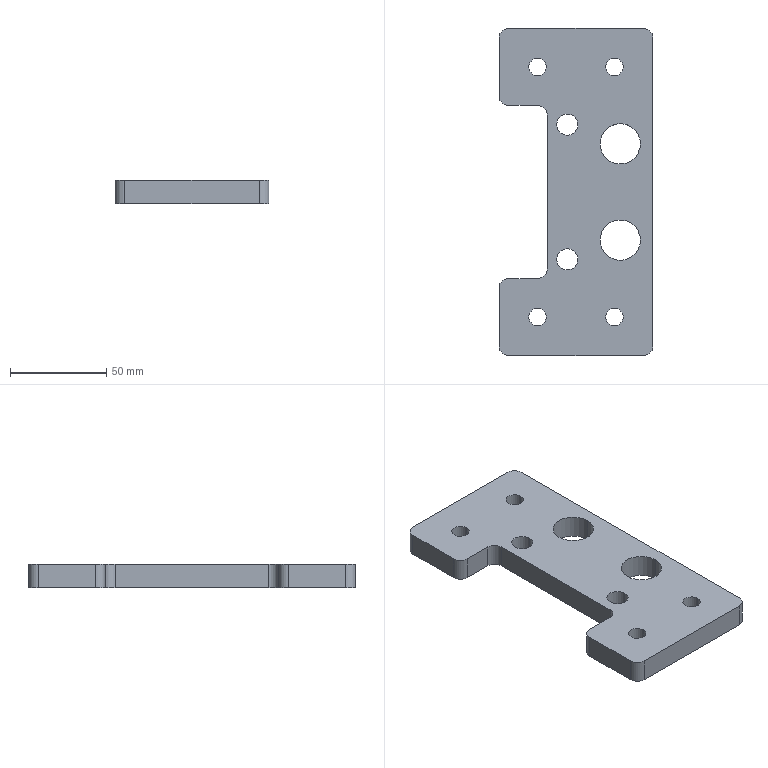Part | SolidWorks | features ICE 2, MoveFace 2, 3DProfileFeature 1, BaseBody 1, Fillet 1, HoleWzd 1 | 1 solid | 34 faces | box 80 x 170 x 12 mm | volume 122295 mm3 | cylinder 24 | plane 10 | commonest cylinder face diameters 9 x8 10 x8 11 x4 21 x4
STEP:
#1=CARTESIAN_POINT('',(33.5,25.,0.));
#2=VERTEX_POINT('',#1);
#3=CARTESIAN_POINT('',(12.5,25.,0.));
#4=VERTEX_POINT('',#3);
#5=CARTESIAN_POINT('',(23.,25.,0.));
#6=DIRECTION('',(0.,0.,-1.));
#7=DIRECTION('',(1.,0.,0.));
#8=AXIS2_PLACEMENT_3D('',#5,#6,#7);
#9=CIRCLE('',#8,10.5);
#10=EDGE_CURVE('',#2,#4,#9,.T.);
#11=ORIENTED_EDGE('',*,*,#10,.T.);
#12=CARTESIAN_POINT('',(12.5,25.,12.));
#13=VERTEX_POINT('',#12);
#14=CARTESIAN_POINT('',(12.5,25.,-0.001));
#15=DIRECTION('',(0.,0.,1.));
#16=VECTOR('',#15,1000.);
#17=LINE('',#14,#16);
#18=EDGE_CURVE('',#4,#13,#17,.T.);
#19=ORIENTED_EDGE('',*,*,#18,.T.);
#20=CARTESIAN_POINT('',(33.5,25.,12.));
#21=VERTEX_POINT('',#20);
#22=CARTESIAN_POINT('',(23.,25.,12.));
#23=DIRECTION('',(0.,0.,1.));
#24=DIRECTION('',(1.,0.,0.));
#25=AXIS2_PLACEMENT_3D('',#22,#23,#24);
#26=CIRCLE('',#25,10.5);
#27=EDGE_CURVE('',#13,#21,#26,.T.);
#28=ORIENTED_EDGE('',*,*,#27,.T.);
#29=CARTESIAN_POINT('',(33.5,25.,-0.001));
#30=DIRECTION('',(0.,0.,1.));
#31=VECTOR('',#30,1000.);
#32=LINE('',#29,#31);
#33=EDGE_CURVE('',#2,#21,#32,.T.);
#34=ORIENTED_EDGE('',*,*,#33,.F.);
#35=EDGE_LOOP('',(#11,#19,#28,#34));
#36=FACE_OUTER_BOUND('',#35,.T.);
#37=CARTESIAN_POINT('',(23.,25.,-0.001));
#38=DIRECTION('',(0.,0.,1.));
#39=DIRECTION('',(1.,0.,0.));
#40=AXIS2_PLACEMENT_3D('',#37,#38,#39);
#41=CYLINDRICAL_SURFACE('',#40,10.5);
#42=ADVANCED_FACE('',(#36),#41,.F.);
#43=CARTESIAN_POINT('',(33.5,-25.,0.));
#44=VERTEX_POINT('',#43);
#45=CARTESIAN_POINT('',(12.5,-25.,0.));
#46=VERTEX_POINT('',#45);
#47=CARTESIAN_POINT('',(23.,-25.,0.));
#48=DIRECTION('',(0.,0.,-1.));
#49=DIRECTION('',(1.,0.,0.));
#50=AXIS2_PLACEMENT_3D('',#47,#48,#49);
#51=CIRCLE('',#50,10.5);
#52=EDGE_CURVE('',#44,#46,#51,.T.);
#53=ORIENTED_EDGE('',*,*,#52,.T.);
#54=CARTESIAN_POINT('',(12.5,-25.,12.));
#55=VERTEX_POINT('',#54);
#56=CARTESIAN_POINT('',(12.5,-25.,-0.001));
#57=DIRECTION('',(0.,0.,1.));
#58=VECTOR('',#57,1000.);
#59=LINE('',#56,#58);
#60=EDGE_CURVE('',#46,#55,#59,.T.);
#61=ORIENTED_EDGE('',*,*,#60,.T.);
#62=CARTESIAN_POINT('',(33.5,-25.,12.));
#63=VERTEX_POINT('',#62);
#64=CARTESIAN_POINT('',(23.,-25.,12.));
#65=DIRECTION('',(0.,0.,1.));
#66=DIRECTION('',(1.,0.,0.));
#67=AXIS2_PLACEMENT_3D('',#64,#65,#66);
#68=CIRCLE('',#67,10.5);
#69=EDGE_CURVE('',#55,#63,#68,.T.);
#70=ORIENTED_EDGE('',*,*,#69,.T.);
#71=CARTESIAN_POINT('',(33.5,-25.,-0.001));
#72=DIRECTION('',(0.,0.,1.));
#73=VECTOR('',#72,1000.);
#74=LINE('',#71,#73);
#75=EDGE_CURVE('',#44,#63,#74,.T.);
#76=ORIENTED_EDGE('',*,*,#75,.F.);
#77=EDGE_LOOP('',(#53,#61,#70,#76));
#78=FACE_OUTER_BOUND('',#77,.T.);
#79=CARTESIAN_POINT('',(23.,-25.,-0.001));
#80=DIRECTION('',(0.,0.,1.));
#81=DIRECTION('',(1.,0.,0.));
#82=AXIS2_PLACEMENT_3D('',#79,#80,#81);
#83=CYLINDRICAL_SURFACE('',#82,10.5);
#84=ADVANCED_FACE('',(#78),#83,.F.);
#85=CARTESIAN_POINT('',(-10.,35.,0.));
#86=VERTEX_POINT('',#85);
#87=CARTESIAN_POINT('',(1.,35.,0.));
#88=VERTEX_POINT('',#87);
#89=CARTESIAN_POINT('',(-4.5,35.,0.));
#90=DIRECTION('',(0.,0.,1.));
#91=DIRECTION('',(1.,0.,0.));
#92=AXIS2_PLACEMENT_3D('',#89,#90,#91);
#93=CIRCLE('',#92,5.5);
#94=EDGE_CURVE('',#86,#88,#93,.T.);
#95=ORIENTED_EDGE('',*,*,#94,.F.);
#96=CARTESIAN_POINT('',(-10.,35.,12.));
#97=VERTEX_POINT('',#96);
#98=CARTESIAN_POINT('',(-10.,35.,10.));
#99=DIRECTION('',(0.,0.,1.));
#100=VECTOR('',#99,1000.);
#101=LINE('',#98,#100);
#102=EDGE_CURVE('',#86,#97,#101,.T.);
#103=ORIENTED_EDGE('',*,*,#102,.T.);
#104=CARTESIAN_POINT('',(1.,35.,12.));
#105=VERTEX_POINT('',#104);
#106=CARTESIAN_POINT('',(-4.5,35.,12.));
#107=DIRECTION('',(0.,0.,1.));
#108=DIRECTION('',(1.,0.,0.));
#109=AXIS2_PLACEMENT_3D('',#106,#107,#108);
#110=CIRCLE('',#109,5.5);
#111=EDGE_CURVE('',#97,#105,#110,.T.);
#112=ORIENTED_EDGE('',*,*,#111,.T.);
#113=CARTESIAN_POINT('',(1.,35.,10.));
#114=DIRECTION('',(0.,0.,1.));
#115=VECTOR('',#114,1000.);
#116=LINE('',#113,#115);
#117=EDGE_CURVE('',#88,#105,#116,.T.);
#118=ORIENTED_EDGE('',*,*,#117,.F.);
#119=EDGE_LOOP('',(#95,#103,#112,#118));
#120=FACE_OUTER_BOUND('',#119,.T.);
#121=CARTESIAN_POINT('',(-4.5,35.,10.));
#122=DIRECTION('',(0.,0.,1.));
#123=DIRECTION('',(1.,0.,0.));
#124=AXIS2_PLACEMENT_3D('',#121,#122,#123);
#125=CYLINDRICAL_SURFACE('',#124,5.5);
#126=ADVANCED_FACE('',(#120),#125,.F.);
#127=CARTESIAN_POINT('',(-10.,-35.,0.));
#128=VERTEX_POINT('',#127);
#129=CARTESIAN_POINT('',(1.,-35.,0.));
#130=VERTEX_POINT('',#129);
#131=CARTESIAN_POINT('',(-4.5,-35.,0.));
#132=DIRECTION('',(0.,0.,1.));
#133=DIRECTION('',(1.,0.,0.));
#134=AXIS2_PLACEMENT_3D('',#131,#132,#133);
#135=CIRCLE('',#134,5.5);
#136=EDGE_CURVE('',#128,#130,#135,.T.);
#137=ORIENTED_EDGE('',*,*,#136,.F.);
#138=CARTESIAN_POINT('',(-10.,-35.,12.));
#139=VERTEX_POINT('',#138);
#140=CARTESIAN_POINT('',(-10.,-35.,10.));
#141=DIRECTION('',(0.,0.,1.));
#142=VECTOR('',#141,1000.);
#143=LINE('',#140,#142);
#144=EDGE_CURVE('',#128,#139,#143,.T.);
#145=ORIENTED_EDGE('',*,*,#144,.T.);
#146=CARTESIAN_POINT('',(1.,-35.,12.));
#147=VERTEX_POINT('',#146);
#148=CARTESIAN_POINT('',(-4.5,-35.,12.));
#149=DIRECTION('',(0.,0.,1.));
#150=DIRECTION('',(1.,0.,0.));
#151=AXIS2_PLACEMENT_3D('',#148,#149,#150);
#152=CIRCLE('',#151,5.5);
#153=EDGE_CURVE('',#139,#147,#152,.T.);
#154=ORIENTED_EDGE('',*,*,#153,.T.);
#155=CARTESIAN_POINT('',(1.,-35.,10.));
#156=DIRECTION('',(0.,0.,1.));
#157=VECTOR('',#156,1000.);
#158=LINE('',#155,#157);
#159=EDGE_CURVE('',#130,#147,#158,.T.);
#160=ORIENTED_EDGE('',*,*,#159,.F.);
#161=EDGE_LOOP('',(#137,#145,#154,#160));
#162=FACE_OUTER_BOUND('',#161,.T.);
#163=CARTESIAN_POINT('',(-4.5,-35.,10.));
#164=DIRECTION('',(0.,0.,1.));
#165=DIRECTION('',(1.,0.,0.));
#166=AXIS2_PLACEMENT_3D('',#163,#164,#165);
#167=CYLINDRICAL_SURFACE('',#166,5.5);
#168=ADVANCED_FACE('',(#162),#167,.F.);
#169=CARTESIAN_POINT('',(-24.5,65.,0.));
#170=VERTEX_POINT('',#169);
#171=CARTESIAN_POINT('',(-15.5,65.,0.));
#172=VERTEX_POINT('',#171);
#173=CARTESIAN_POINT('',(-20.,65.,0.));
#174=DIRECTION('',(0.,0.,1.));
#175=DIRECTION('',(1.,0.,0.));
#176=AXIS2_PLACEMENT_3D('',#173,#174,#175);
#177=CIRCLE('',#176,4.5);
#178=EDGE_CURVE('',#170,#172,#177,.T.);
#179=ORIENTED_EDGE('',*,*,#178,.F.);
#180=CARTESIAN_POINT('',(-24.5,65.,12.));
#181=VERTEX_POINT('',#180);
#182=CARTESIAN_POINT('',(-24.5,65.,10.));
#183=DIRECTION('',(0.,0.,1.));
#184=VECTOR('',#183,1000.);
#185=LINE('',#182,#184);
#186=EDGE_CURVE('',#170,#181,#185,.T.);
#187=ORIENTED_EDGE('',*,*,#186,.T.);
#188=CARTESIAN_POINT('',(-15.5,65.,12.));
#189=VERTEX_POINT('',#188);
#190=CARTESIAN_POINT('',(-20.,65.,12.));
#191=DIRECTION('',(0.,0.,1.));
#192=DIRECTION('',(1.,0.,0.));
#193=AXIS2_PLACEMENT_3D('',#190,#191,#192);
#194=CIRCLE('',#193,4.5);
#195=EDGE_CURVE('',#181,#189,#194,.T.);
#196=ORIENTED_EDGE('',*,*,#195,.T.);
#197=CARTESIAN_POINT('',(-15.5,65.,10.));
#198=DIRECTION('',(0.,0.,1.));
#199=VECTOR('',#198,1000.);
#200=LINE('',#197,#199);
#201=EDGE_CURVE('',#172,#189,#200,.T.);
#202=ORIENTED_EDGE('',*,*,#201,.F.);
#203=EDGE_LOOP('',(#179,#187,#196,#202));
#204=FACE_OUTER_BOUND('',#203,.T.);
#205=CARTESIAN_POINT('',(-20.,65.,10.));
#206=DIRECTION('',(0.,0.,1.));
#207=DIRECTION('',(1.,0.,0.));
#208=AXIS2_PLACEMENT_3D('',#205,#206,#207);
#209=CYLINDRICAL_SURFACE('',#208,4.5);
#210=ADVANCED_FACE('',(#204),#209,.F.);
#211=CARTESIAN_POINT('',(15.5,65.,0.));
#212=VERTEX_POINT('',#211);
#213=CARTESIAN_POINT('',(24.5,65.,0.));
#214=VERTEX_POINT('',#213);
#215=CARTESIAN_POINT('',(20.,65.,0.));
#216=DIRECTION('',(0.,0.,1.));
#217=DIRECTION('',(1.,0.,0.));
#218=AXIS2_PLACEMENT_3D('',#215,#216,#217);
#219=CIRCLE('',#218,4.5);
#220=EDGE_CURVE('',#212,#214,#219,.T.);
#221=ORIENTED_EDGE('',*,*,#220,.F.);
#222=CARTESIAN_POINT('',(15.5,65.,12.));
#223=VERTEX_POINT('',#222);
#224=CARTESIAN_POINT('',(15.5,65.,10.));
#225=DIRECTION('',(0.,0.,1.));
#226=VECTOR('',#225,1000.);
#227=LINE('',#224,#226);
#228=EDGE_CURVE('',#212,#223,#227,.T.);
#229=ORIENTED_EDGE('',*,*,#228,.T.);
#230=CARTESIAN_POINT('',(24.5,65.,12.));
#231=VERTEX_POINT('',#230);
#232=CARTESIAN_POINT('',(20.,65.,12.));
#233=DIRECTION('',(0.,0.,1.));
#234=DIRECTION('',(1.,0.,0.));
#235=AXIS2_PLACEMENT_3D('',#232,#233,#234);
#236=CIRCLE('',#235,4.5);
#237=EDGE_CURVE('',#223,#231,#236,.T.);
#238=ORIENTED_EDGE('',*,*,#237,.T.);
#239=CARTESIAN_POINT('',(24.5,65.,10.));
#240=DIRECTION('',(0.,0.,1.));
#241=VECTOR('',#240,1000.);
#242=LINE('',#239,#241);
#243=EDGE_CURVE('',#214,#231,#242,.T.);
#244=ORIENTED_EDGE('',*,*,#243,.F.);
#245=EDGE_LOOP('',(#221,#229,#238,#244));
#246=FACE_OUTER_BOUND('',#245,.T.);
#247=CARTESIAN_POINT('',(20.,65.,10.));
#248=DIRECTION('',(0.,0.,1.));
#249=DIRECTION('',(1.,0.,0.));
#250=AXIS2_PLACEMENT_3D('',#247,#248,#249);
#251=CYLINDRICAL_SURFACE('',#250,4.5);
#252=ADVANCED_FACE('',(#246),#251,.F.);
#253=CARTESIAN_POINT('',(-24.5,-65.,0.));
#254=VERTEX_POINT('',#253);
#255=CARTESIAN_POINT('',(-15.5,-65.,0.));
#256=VERTEX_POINT('',#255);
#257=CARTESIAN_POINT('',(-20.,-65.,0.));
#258=DIRECTION('',(0.,0.,1.));
#259=DIRECTION('',(1.,0.,0.));
#260=AXIS2_PLACEMENT_3D('',#257,#258,#259);
#261=CIRCLE('',#260,4.5);
#262=EDGE_CURVE('',#254,#256,#261,.T.);
#263=ORIENTED_EDGE('',*,*,#262,.F.);
#264=CARTESIAN_POINT('',(-24.5,-65.,12.));
#265=VERTEX_POINT('',#264);
#266=CARTESIAN_POINT('',(-24.5,-65.,10.));
#267=DIRECTION('',(0.,0.,1.));
#268=VECTOR('',#267,1000.);
#269=LINE('',#266,#268);
#270=EDGE_CURVE('',#254,#265,#269,.T.);
#271=ORIENTED_EDGE('',*,*,#270,.T.);
#272=CARTESIAN_POINT('',(-15.5,-65.,12.));
#273=VERTEX_POINT('',#272);
#274=CARTESIAN_POINT('',(-20.,-65.,12.));
#275=DIRECTION('',(0.,0.,1.));
#276=DIRECTION('',(1.,0.,0.));
#277=AXIS2_PLACEMENT_3D('',#274,#275,#276);
#278=CIRCLE('',#277,4.5);
#279=EDGE_CURVE('',#265,#273,#278,.T.);
#280=ORIENTED_EDGE('',*,*,#279,.T.);
#281=CARTESIAN_POINT('',(-15.5,-65.,10.));
#282=DIRECTION('',(0.,0.,1.));
#283=VECTOR('',#282,1000.);
#284=LINE('',#281,#283);
#285=EDGE_CURVE('',#256,#273,#284,.T.);
#286=ORIENTED_EDGE('',*,*,#285,.F.);
#287=EDGE_LOOP('',(#263,#271,#280,#286));
#288=FACE_OUTER_BOUND('',#287,.T.);
#289=CARTESIAN_POINT('',(-20.,-65.,10.));
#290=DIRECTION('',(0.,0.,1.));
#291=DIRECTION('',(1.,0.,0.));
#292=AXIS2_PLACEMENT_3D('',#289,#290,#291);
#293=CYLINDRICAL_SURFACE('',#292,4.5);
#294=ADVANCED_FACE('',(#288),#293,.F.);
#295=CARTESIAN_POINT('',(15.5,-65.,0.));
#296=VERTEX_POINT('',#295);
#297=CARTESIAN_POINT('',(24.5,-65.,0.));
#298=VERTEX_POINT('',#297);
#299=CARTESIAN_POINT('',(20.,-65.,0.));
#300=DIRECTION('',(0.,0.,1.));
#301=DIRECTION('',(1.,0.,0.));
#302=AXIS2_PLACEMENT_3D('',#299,#300,#301);
#303=CIRCLE('',#302,4.5);
#304=EDGE_CURVE('',#296,#298,#303,.T.);
#305=ORIENTED_EDGE('',*,*,#304,.F.);
#306=CARTESIAN_POINT('',(15.5,-65.,12.));
#307=VERTEX_POINT('',#306);
#308=CARTESIAN_POINT('',(15.5,-65.,10.));
#309=DIRECTION('',(0.,0.,1.));
#310=VECTOR('',#309,1000.);
#311=LINE('',#308,#310);
#312=EDGE_CURVE('',#296,#307,#311,.T.);
#313=ORIENTED_EDGE('',*,*,#312,.T.);
#314=CARTESIAN_POINT('',(24.5,-65.,12.));
#315=VERTEX_POINT('',#314);
#316=CARTESIAN_POINT('',(20.,-65.,12.));
#317=DIRECTION('',(0.,0.,1.));
#318=DIRECTION('',(1.,0.,0.));
#319=AXIS2_PLACEMENT_3D('',#316,#317,#318);
#320=CIRCLE('',#319,4.5);
#321=EDGE_CURVE('',#307,#315,#320,.T.);
#322=ORIENTED_EDGE('',*,*,#321,.T.);
#323=CARTESIAN_POINT('',(24.5,-65.,10.));
#324=DIRECTION('',(0.,0.,1.));
#325=VECTOR('',#324,1000.);
#326=LINE('',#323,#325);
#327=EDGE_CURVE('',#298,#315,#326,.T.);
#328=ORIENTED_EDGE('',*,*,#327,.F.);
#329=EDGE_LOOP('',(#305,#313,#322,#328));
#330=FACE_OUTER_BOUND('',#329,.T.);
#331=CARTESIAN_POINT('',(20.,-65.,10.));
#332=DIRECTION('',(0.,0.,1.));
#333=DIRECTION('',(1.,0.,0.));
#334=AXIS2_PLACEMENT_3D('',#331,#332,#333);
#335=CYLINDRICAL_SURFACE('',#334,4.5);
#336=ADVANCED_FACE('',(#330),#335,.F.);
#337=CARTESIAN_POINT('',(-40.,80.,0.));
#338=VERTEX_POINT('',#337);
#339=CARTESIAN_POINT('',(-40.,50.,0.));
#340=VERTEX_POINT('',#339);
#341=CARTESIAN_POINT('',(-40.,85.,0.));
#342=DIRECTION('',(0.,-1.,0.));
#343=VECTOR('',#342,1000.);
#344=LINE('',#341,#343);
#345=EDGE_CURVE('',#338,#340,#344,.T.);
#346=ORIENTED_EDGE('',*,*,#345,.T.);
#347=CARTESIAN_POINT('',(-40.,50.,12.));
#348=VERTEX_POINT('',#347);
#349=CARTESIAN_POINT('',(-40.,50.,10.));
#350=DIRECTION('',(0.,0.,1.));
#351=VECTOR('',#350,1000.);
#352=LINE('',#349,#351);
#353=EDGE_CURVE('',#340,#348,#352,.T.);
#354=ORIENTED_EDGE('',*,*,#353,.T.);
#355=CARTESIAN_POINT('',(-40.,80.,12.));
#356=VERTEX_POINT('',#355);
#357=CARTESIAN_POINT('',(-40.,85.,12.));
#358=DIRECTION('',(0.,-1.,0.));
#359=VECTOR('',#358,1000.);
#360=LINE('',#357,#359);
#361=EDGE_CURVE('',#356,#348,#360,.T.);
#362=ORIENTED_EDGE('',*,*,#361,.F.);
#363=CARTESIAN_POINT('',(-40.,80.,10.));
#364=DIRECTION('',(0.,0.,-1.));
#365=VECTOR('',#364,1000.);
#366=LINE('',#363,#365);
#367=EDGE_CURVE('',#356,#338,#366,.T.);
#368=ORIENTED_EDGE('',*,*,#367,.T.);
#369=EDGE_LOOP('',(#346,#354,#362,#368));
#370=FACE_OUTER_BOUND('',#369,.T.);
#371=CARTESIAN_POINT('',(-40.,85.,10.));
#372=DIRECTION('',(1.,0.,0.));
#373=DIRECTION('',(0.,1.,0.));
#374=AXIS2_PLACEMENT_3D('',#371,#372,#373);
#375=PLANE('',#374);
#376=ADVANCED_FACE('',(#370),#375,.F.);
#377=CARTESIAN_POINT('',(-35.,85.,12.));
#378=VERTEX_POINT('',#377);
#379=CARTESIAN_POINT('',(-35.,80.,12.));
#380=DIRECTION('',(0.,0.,1.));
#381=DIRECTION('',(1.,0.,0.));
#382=AXIS2_PLACEMENT_3D('',#379,#380,#381);
#383=CIRCLE('',#382,5.);
#384=EDGE_CURVE('',#378,#356,#383,.T.);
#385=ORIENTED_EDGE('',*,*,#384,.F.);
#386=CARTESIAN_POINT('',(-35.,85.,0.));
#387=VERTEX_POINT('',#386);
#388=CARTESIAN_POINT('',(-35.,85.,10.));
#389=DIRECTION('',(0.,0.,1.));
#390=VECTOR('',#389,1000.);
#391=LINE('',#388,#390);
#392=EDGE_CURVE('',#387,#378,#391,.T.);
#393=ORIENTED_EDGE('',*,*,#392,.F.);
#394=CARTESIAN_POINT('',(-35.,80.,0.));
#395=DIRECTION('',(0.,0.,-1.));
#396=DIRECTION('',(1.,0.,0.));
#397=AXIS2_PLACEMENT_3D('',#394,#395,#396);
#398=CIRCLE('',#397,5.);
#399=EDGE_CURVE('',#338,#387,#398,.T.);
#400=ORIENTED_EDGE('',*,*,#399,.F.);
#401=ORIENTED_EDGE('',*,*,#367,.F.);
#402=EDGE_LOOP('',(#385,#393,#400,#401));
#403=FACE_OUTER_BOUND('',#402,.T.);
#404=CARTESIAN_POINT('',(-35.,80.,10.));
#405=DIRECTION('',(0.,0.,-1.));
#406=DIRECTION('',(-1.,0.,0.));
#407=AXIS2_PLACEMENT_3D('',#404,#405,#406);
#408=CYLINDRICAL_SURFACE('',#407,5.);
#409=ADVANCED_FACE('',(#403),#408,.T.);
#410=CARTESIAN_POINT('',(40.,80.,12.));
#411=VERTEX_POINT('',#410);
#412=CARTESIAN_POINT('',(35.,85.,12.));
#413=VERTEX_POINT('',#412);
#414=CARTESIAN_POINT('',(35.,80.,12.));
#415=DIRECTION('',(0.,0.,1.));
#416=DIRECTION('',(1.,0.,0.));
#417=AXIS2_PLACEMENT_3D('',#414,#415,#416);
#418=CIRCLE('',#417,5.);
#419=EDGE_CURVE('',#411,#413,#418,.T.);
#420=ORIENTED_EDGE('',*,*,#419,.F.);
#421=CARTESIAN_POINT('',(40.,80.,0.));
#422=VERTEX_POINT('',#421);
#423=CARTESIAN_POINT('',(40.,80.,10.));
#424=DIRECTION('',(0.,0.,1.));
#425=VECTOR('',#424,1000.);
#426=LINE('',#423,#425);
#427=EDGE_CURVE('',#422,#411,#426,.T.);
#428=ORIENTED_EDGE('',*,*,#427,.F.);
#429=CARTESIAN_POINT('',(35.,85.,0.));
#430=VERTEX_POINT('',#429);
#431=CARTESIAN_POINT('',(35.,80.,0.));
#432=DIRECTION('',(0.,0.,-1.));
#433=DIRECTION('',(1.,0.,0.));
#434=AXIS2_PLACEMENT_3D('',#431,#432,#433);
#435=CIRCLE('',#434,5.);
#436=EDGE_CURVE('',#430,#422,#435,.T.);
#437=ORIENTED_EDGE('',*,*,#436,.F.);
#438=CARTESIAN_POINT('',(35.,85.,10.));
#439=DIRECTION('',(0.,0.,-1.));
#440=VECTOR('',#439,1000.);
#441=LINE('',#438,#440);
#442=EDGE_CURVE('',#413,#430,#441,.T.);
#443=ORIENTED_EDGE('',*,*,#442,.F.);
#444=EDGE_LOOP('',(#420,#428,#437,#443));
#445=FACE_OUTER_BOUND('',#444,.T.);
#446=CARTESIAN_POINT('',(35.,80.,10.));
#447=DIRECTION('',(0.,0.,-1.));
#448=DIRECTION('',(-1.,0.,0.));
#449=AXIS2_PLACEMENT_3D('',#446,#447,#448);
#450=CYLINDRICAL_SURFACE('',#449,5.);
#451=ADVANCED_FACE('',(#445),#450,.T.);
#452=CARTESIAN_POINT('',(35.,-85.,12.));
#453=VERTEX_POINT('',#452);
#454=CARTESIAN_POINT('',(40.,-80.,12.));
#455=VERTEX_POINT('',#454);
#456=CARTESIAN_POINT('',(35.,-80.,12.));
#457=DIRECTION('',(0.,0.,1.));
#458=DIRECTION('',(1.,0.,0.));
#459=AXIS2_PLACEMENT_3D('',#456,#457,#458);
#460=CIRCLE('',#459,5.);
#461=EDGE_CURVE('',#453,#455,#460,.T.);
#462=ORIENTED_EDGE('',*,*,#461,.F.);
#463=CARTESIAN_POINT('',(35.,-85.,0.));
#464=VERTEX_POINT('',#463);
#465=CARTESIAN_POINT('',(35.,-85.,10.));
#466=DIRECTION('',(0.,0.,1.));
#467=VECTOR('',#466,1000.);
#468=LINE('',#465,#467);
#469=EDGE_CURVE('',#464,#453,#468,.T.);
#470=ORIENTED_EDGE('',*,*,#469,.F.);
#471=CARTESIAN_POINT('',(40.,-80.,0.));
#472=VERTEX_POINT('',#471);
#473=CARTESIAN_POINT('',(35.,-80.,0.));
#474=DIRECTION('',(0.,0.,-1.));
#475=DIRECTION('',(1.,0.,0.));
#476=AXIS2_PLACEMENT_3D('',#473,#474,#475);
#477=CIRCLE('',#476,5.);
#478=EDGE_CURVE('',#472,#464,#477,.T.);
#479=ORIENTED_EDGE('',*,*,#478,.F.);
#480=CARTESIAN_POINT('',(40.,-80.,10.));
#481=DIRECTION('',(0.,0.,-1.));
#482=VECTOR('',#481,1000.);
#483=LINE('',#480,#482);
#484=EDGE_CURVE('',#455,#472,#483,.T.);
#485=ORIENTED_EDGE('',*,*,#484,.F.);
#486=EDGE_LOOP('',(#462,#470,#479,#485));
#487=FACE_OUTER_BOUND('',#486,.T.);
#488=CARTESIAN_POINT('',(35.,-80.,10.));
#489=DIRECTION('',(0.,0.,-1.));
#490=DIRECTION('',(-1.,0.,0.));
#491=AXIS2_PLACEMENT_3D('',#488,#489,#490);
#492=CYLINDRICAL_SURFACE('',#491,5.);
#493=ADVANCED_FACE('',(#487),#492,.T.);
#494=CARTESIAN_POINT('',(-40.,-80.,12.));
#495=VERTEX_POINT('',#494);
#496=CARTESIAN_POINT('',(-35.,-85.,12.));
#497=VERTEX_POINT('',#496);
#498=CARTESIAN_POINT('',(-35.,-80.,12.));
#499=DIRECTION('',(0.,0.,1.));
#500=DIRECTION('',(1.,0.,0.));
#501=AXIS2_PLACEMENT_3D('',#498,#499,#500);
#502=CIRCLE('',#501,5.);
#503=EDGE_CURVE('',#495,#497,#502,.T.);
#504=ORIENTED_EDGE('',*,*,#503,.F.);
#505=CARTESIAN_POINT('',(-40.,-80.,0.));
#506=VERTEX_POINT('',#505);
#507=CARTESIAN_POINT('',(-40.,-80.,10.));
#508=DIRECTION('',(0.,0.,1.));
#509=VECTOR('',#508,1000.);
#510=LINE('',#507,#509);
#511=EDGE_CURVE('',#506,#495,#510,.T.);
#512=ORIENTED_EDGE('',*,*,#511,.F.);
#513=CARTESIAN_POINT('',(-35.,-85.,0.));
#514=VERTEX_POINT('',#513);
#515=CARTESIAN_POINT('',(-35.,-80.,0.));
#516=DIRECTION('',(0.,0.,-1.));
#517=DIRECTION('',(1.,0.,0.));
#518=AXIS2_PLACEMENT_3D('',#515,#516,#517);
#519=CIRCLE('',#518,5.);
#520=EDGE_CURVE('',#514,#506,#519,.T.);
#521=ORIENTED_EDGE('',*,*,#520,.F.);
#522=CARTESIAN_POINT('',(-35.,-85.,10.));
#523=DIRECTION('',(0.,0.,-1.));
#524=VECTOR('',#523,1000.);
#525=LINE('',#522,#524);
#526=EDGE_CURVE('',#497,#514,#525,.T.);
#527=ORIENTED_EDGE('',*,*,#526,.F.);
#528=EDGE_LOOP('',(#504,#512,#521,#527));
#529=FACE_OUTER_BOUND('',#528,.T.);
#530=CARTESIAN_POINT('',(-35.,-80.,10.));
#531=DIRECTION('',(0.,0.,-1.));
#532=DIRECTION('',(-1.,0.,0.));
#533=AXIS2_PLACEMENT_3D('',#530,#531,#532);
#534=CYLINDRICAL_SURFACE('',#533,5.);
#535=ADVANCED_FACE('',(#529),#534,.T.);
#536=ORIENTED_EDGE('',*,*,#10,.F.);
#537=CARTESIAN_POINT('',(23.,25.,0.));
#538=DIRECTION('',(0.,0.,-1.));
#539=DIRECTION('',(1.,0.,0.));
#540=AXIS2_PLACEMENT_3D('',#537,#538,#539);
#541=CIRCLE('',#540,10.5);
#542=EDGE_CURVE('',#4,#2,#541,.T.);
#543=ORIENTED_EDGE('',*,*,#542,.F.);
#544=EDGE_LOOP('',(#536,#543));
#545=FACE_BOUND('',#544,.T.);
#546=ORIENTED_EDGE('',*,*,#52,.F.);
#547=CARTESIAN_POINT('',(23.,-25.,0.));
#548=DIRECTION('',(0.,0.,-1.));
#549=DIRECTION('',(1.,0.,0.));
#550=AXIS2_PLACEMENT_3D('',#547,#548,#549);
#551=CIRCLE('',#550,10.5);
#552=EDGE_CURVE('',#46,#44,#551,.T.);
#553=ORIENTED_EDGE('',*,*,#552,.F.);
#554=EDGE_LOOP('',(#546,#553));
#555=FACE_BOUND('',#554,.T.);
#556=CARTESIAN_POINT('',(20.,-65.,0.));
#557=DIRECTION('',(0.,0.,1.));
#558=DIRECTION('',(1.,0.,0.));
#559=AXIS2_PLACEMENT_3D('',#556,#557,#558);
#560=CIRCLE('',#559,4.5);
#561=EDGE_CURVE('',#298,#296,#560,.T.);
#562=ORIENTED_EDGE('',*,*,#561,.T.);
#563=ORIENTED_EDGE('',*,*,#304,.T.);
#564=EDGE_LOOP('',(#562,#563));
#565=FACE_BOUND('',#564,.T.);
#566=CARTESIAN_POINT('',(-20.,-65.,0.));
#567=DIRECTION('',(0.,0.,1.));
#568=DIRECTION('',(1.,0.,0.));
#569=AXIS2_PLACEMENT_3D('',#566,#567,#568);
#570=CIRCLE('',#569,4.5);
#571=EDGE_CURVE('',#256,#254,#570,.T.);
#572=ORIENTED_EDGE('',*,*,#571,.T.);
#573=ORIENTED_EDGE('',*,*,#262,.T.);
#574=EDGE_LOOP('',(#572,#573));
#575=FACE_BOUND('',#574,.T.);
#576=CARTESIAN_POINT('',(20.,65.,0.));
#577=DIRECTION('',(0.,0.,1.));
#578=DIRECTION('',(1.,0.,0.));
#579=AXIS2_PLACEMENT_3D('',#576,#577,#578);
#580=CIRCLE('',#579,4.5);
#581=EDGE_CURVE('',#214,#212,#580,.T.);
#582=ORIENTED_EDGE('',*,*,#581,.T.);
#583=ORIENTED_EDGE('',*,*,#220,.T.);
#584=EDGE_LOOP('',(#582,#583));
#585=FACE_BOUND('',#584,.T.);
#586=CARTESIAN_POINT('',(-20.,65.,0.));
#587=DIRECTION('',(0.,0.,1.));
#588=DIRECTION('',(1.,0.,0.));
#589=AXIS2_PLACEMENT_3D('',#586,#587,#588);
#590=CIRCLE('',#589,4.5);
#591=EDGE_CURVE('',#172,#170,#590,.T.);
#592=ORIENTED_EDGE('',*,*,#591,.T.);
#593=ORIENTED_EDGE('',*,*,#178,.T.);
#594=EDGE_LOOP('',(#592,#593));
#595=FACE_BOUND('',#594,.T.);
#596=CARTESIAN_POINT('',(-4.5,-35.,0.));
#597=DIRECTION('',(0.,0.,1.));
#598=DIRECTION('',(1.,0.,0.));
#599=AXIS2_PLACEMENT_3D('',#596,#597,#598);
#600=CIRCLE('',#599,5.5);
#601=EDGE_CURVE('',#130,#128,#600,.T.);
#602=ORIENTED_EDGE('',*,*,#601,.T.);
#603=ORIENTED_EDGE('',*,*,#136,.T.);
#604=EDGE_LOOP('',(#602,#603));
#605=FACE_BOUND('',#604,.T.);
#606=CARTESIAN_POINT('',(-4.5,35.,0.));
#607=DIRECTION('',(0.,0.,1.));
#608=DIRECTION('',(1.,0.,0.));
#609=AXIS2_PLACEMENT_3D('',#606,#607,#608);
#610=CIRCLE('',#609,5.5);
#611=EDGE_CURVE('',#88,#86,#610,.T.);
#612=ORIENTED_EDGE('',*,*,#611,.T.);
#613=ORIENTED_EDGE('',*,*,#94,.T.);
#614=EDGE_LOOP('',(#612,#613));
#615=FACE_BOUND('',#614,.T.);
#616=CARTESIAN_POINT('',(-40.,-50.,0.));
#617=VERTEX_POINT('',#616);
#618=CARTESIAN_POINT('',(-40.,85.,0.));
#619=DIRECTION('',(0.,-1.,0.));
#620=VECTOR('',#619,1000.);
#621=LINE('',#618,#620);
#622=EDGE_CURVE('',#617,#506,#621,.T.);
#623=ORIENTED_EDGE('',*,*,#622,.F.);
#624=CARTESIAN_POINT('',(-35.,-45.,0.));
#625=VERTEX_POINT('',#624);
#626=CARTESIAN_POINT('',(-35.,-50.,0.));
#627=DIRECTION('',(0.,0.,-1.));
#628=DIRECTION('',(1.,0.,0.));
#629=AXIS2_PLACEMENT_3D('',#626,#627,#628);
#630=CIRCLE('',#629,5.);
#631=EDGE_CURVE('',#617,#625,#630,.T.);
#632=ORIENTED_EDGE('',*,*,#631,.T.);
#633=CARTESIAN_POINT('',(-20.,-45.,0.));
#634=VERTEX_POINT('',#633);
#635=CARTESIAN_POINT('',(-15.,-45.,0.));
#636=DIRECTION('',(-1.,0.,0.));
#637=VECTOR('',#636,1000.);
#638=LINE('',#635,#637);
#639=EDGE_CURVE('',#634,#625,#638,.T.);
#640=ORIENTED_EDGE('',*,*,#639,.F.);
#641=CARTESIAN_POINT('',(-15.,-40.,0.));
#642=VERTEX_POINT('',#641);
#643=CARTESIAN_POINT('',(-20.,-40.,0.));
#644=DIRECTION('',(0.,0.,1.));
#645=DIRECTION('',(1.,0.,0.));
#646=AXIS2_PLACEMENT_3D('',#643,#644,#645);
#647=CIRCLE('',#646,5.);
#648=EDGE_CURVE('',#634,#642,#647,.T.);
#649=ORIENTED_EDGE('',*,*,#648,.T.);
#650=CARTESIAN_POINT('',(-15.,40.,0.));
#651=VERTEX_POINT('',#650);
#652=CARTESIAN_POINT('',(-15.,45.,0.));
#653=DIRECTION('',(0.,-1.,0.));
#654=VECTOR('',#653,1000.);
#655=LINE('',#652,#654);
#656=EDGE_CURVE('',#651,#642,#655,.T.);
#657=ORIENTED_EDGE('',*,*,#656,.F.);
#658=CARTESIAN_POINT('',(-20.,45.,0.));
#659=VERTEX_POINT('',#658);
#660=CARTESIAN_POINT('',(-20.,40.,0.));
#661=DIRECTION('',(0.,0.,1.));
#662=DIRECTION('',(1.,0.,0.));
#663=AXIS2_PLACEMENT_3D('',#660,#661,#662);
#664=CIRCLE('',#663,5.);
#665=EDGE_CURVE('',#651,#659,#664,.T.);
#666=ORIENTED_EDGE('',*,*,#665,.T.);
#667=CARTESIAN_POINT('',(-35.,45.,0.));
#668=VERTEX_POINT('',#667);
#669=CARTESIAN_POINT('',(-40.,45.,0.));
#670=DIRECTION('',(1.,0.,0.));
#671=VECTOR('',#670,1000.);
#672=LINE('',#669,#671);
#673=EDGE_CURVE('',#668,#659,#672,.T.);
#674=ORIENTED_EDGE('',*,*,#673,.F.);
#675=CARTESIAN_POINT('',(-35.,50.,0.));
#676=DIRECTION('',(0.,0.,-1.));
#677=DIRECTION('',(1.,0.,0.));
#678=AXIS2_PLACEMENT_3D('',#675,#676,#677);
#679=CIRCLE('',#678,5.);
#680=EDGE_CURVE('',#668,#340,#679,.T.);
#681=ORIENTED_EDGE('',*,*,#680,.T.);
#682=ORIENTED_EDGE('',*,*,#345,.F.);
#683=ORIENTED_EDGE('',*,*,#399,.T.);
#684=CARTESIAN_POINT('',(-40.,85.,0.));
#685=DIRECTION('',(-1.,0.,0.));
#686=VECTOR('',#685,1000.);
#687=LINE('',#684,#686);
#688=EDGE_CURVE('',#430,#387,#687,.T.);
#689=ORIENTED_EDGE('',*,*,#688,.F.);
#690=ORIENTED_EDGE('',*,*,#436,.T.);
#691=CARTESIAN_POINT('',(40.,85.,0.));
#692=DIRECTION('',(0.,1.,0.));
#693=VECTOR('',#692,1000.);
#694=LINE('',#691,#693);
#695=EDGE_CURVE('',#472,#422,#694,.T.);
#696=ORIENTED_EDGE('',*,*,#695,.F.);
#697=ORIENTED_EDGE('',*,*,#478,.T.);
#698=CARTESIAN_POINT('',(-40.,-85.,0.));
#699=DIRECTION('',(1.,0.,0.));
#700=VECTOR('',#699,1000.);
#701=LINE('',#698,#700);
#702=EDGE_CURVE('',#514,#464,#701,.T.);
#703=ORIENTED_EDGE('',*,*,#702,.F.);
#704=ORIENTED_EDGE('',*,*,#520,.T.);
#705=EDGE_LOOP('',(#623,#632,#640,#649,#657,#666,#674,#681,#682,#683,#689,#690,#696,#697,#703,#704));
#706=FACE_OUTER_BOUND('',#705,.T.);
#707=CARTESIAN_POINT('',(0.,0.,0.));
#708=DIRECTION('',(0.,0.,1.));
#709=DIRECTION('',(1.,0.,0.));
#710=AXIS2_PLACEMENT_3D('',#707,#708,#709);
#711=PLANE('',#710);
#712=ADVANCED_FACE('',(#545,#555,#565,#575,#585,#595,#605,#615,#706),#711,.F.);
#713=CARTESIAN_POINT('',(23.,25.,12.));
#714=DIRECTION('',(0.,0.,1.));
#715=DIRECTION('',(1.,0.,0.));
#716=AXIS2_PLACEMENT_3D('',#713,#714,#715);
#717=CIRCLE('',#716,10.5);
#718=EDGE_CURVE('',#21,#13,#717,.T.);
#719=ORIENTED_EDGE('',*,*,#718,.F.);
#720=ORIENTED_EDGE('',*,*,#27,.F.);
#721=EDGE_LOOP('',(#719,#720));
#722=FACE_BOUND('',#721,.T.);
#723=CARTESIAN_POINT('',(23.,-25.,12.));
#724=DIRECTION('',(0.,0.,1.));
#725=DIRECTION('',(1.,0.,0.));
#726=AXIS2_PLACEMENT_3D('',#723,#724,#725);
#727=CIRCLE('',#726,10.5);
#728=EDGE_CURVE('',#63,#55,#727,.T.);
#729=ORIENTED_EDGE('',*,*,#728,.F.);
#730=ORIENTED_EDGE('',*,*,#69,.F.);
#731=EDGE_LOOP('',(#729,#730));
#732=FACE_BOUND('',#731,.T.);
#733=CARTESIAN_POINT('',(-35.,-45.,12.));
#734=VERTEX_POINT('',#733);
#735=CARTESIAN_POINT('',(-20.,-45.,12.));
#736=VERTEX_POINT('',#735);
#737=CARTESIAN_POINT('',(-15.,-45.,12.));
#738=DIRECTION('',(1.,0.,0.));
#739=VECTOR('',#738,1000.);
#740=LINE('',#737,#739);
#741=EDGE_CURVE('',#734,#736,#740,.T.);
#742=ORIENTED_EDGE('',*,*,#741,.F.);
#743=CARTESIAN_POINT('',(-40.,-50.,12.));
#744=VERTEX_POINT('',#743);
#745=CARTESIAN_POINT('',(-35.,-50.,12.));
#746=DIRECTION('',(0.,0.,1.));
#747=DIRECTION('',(1.,0.,0.));
#748=AXIS2_PLACEMENT_3D('',#745,#746,#747);
#749=CIRCLE('',#748,5.);
#750=EDGE_CURVE('',#734,#744,#749,.T.);
#751=ORIENTED_EDGE('',*,*,#750,.T.);
#752=CARTESIAN_POINT('',(-40.,85.,12.));
#753=DIRECTION('',(0.,-1.,0.));
#754=VECTOR('',#753,1000.);
#755=LINE('',#752,#754);
#756=EDGE_CURVE('',#744,#495,#755,.T.);
#757=ORIENTED_EDGE('',*,*,#756,.T.);
#758=ORIENTED_EDGE('',*,*,#503,.T.);
#759=CARTESIAN_POINT('',(-40.,-85.,12.));
#760=DIRECTION('',(1.,0.,0.));
#761=VECTOR('',#760,1000.);
#762=LINE('',#759,#761);
#763=EDGE_CURVE('',#497,#453,#762,.T.);
#764=ORIENTED_EDGE('',*,*,#763,.T.);
#765=ORIENTED_EDGE('',*,*,#461,.T.);
#766=CARTESIAN_POINT('',(40.,85.,12.));
#767=DIRECTION('',(0.,1.,0.));
#768=VECTOR('',#767,1000.);
#769=LINE('',#766,#768);
#770=EDGE_CURVE('',#455,#411,#769,.T.);
#771=ORIENTED_EDGE('',*,*,#770,.T.);
#772=ORIENTED_EDGE('',*,*,#419,.T.);
#773=CARTESIAN_POINT('',(-40.,85.,12.));
#774=DIRECTION('',(-1.,0.,0.));
#775=VECTOR('',#774,1000.);
#776=LINE('',#773,#775);
#777=EDGE_CURVE('',#413,#378,#776,.T.);
#778=ORIENTED_EDGE('',*,*,#777,.T.);
#779=ORIENTED_EDGE('',*,*,#384,.T.);
#780=ORIENTED_EDGE('',*,*,#361,.T.);
#781=CARTESIAN_POINT('',(-35.,45.,12.));
#782=VERTEX_POINT('',#781);
#783=CARTESIAN_POINT('',(-35.,50.,12.));
#784=DIRECTION('',(0.,0.,1.));
#785=DIRECTION('',(1.,0.,0.));
#786=AXIS2_PLACEMENT_3D('',#783,#784,#785);
#787=CIRCLE('',#786,5.);
#788=EDGE_CURVE('',#348,#782,#787,.T.);
#789=ORIENTED_EDGE('',*,*,#788,.T.);
#790=CARTESIAN_POINT('',(-20.,45.,12.));
#791=VERTEX_POINT('',#790);
#792=CARTESIAN_POINT('',(-40.,45.,12.));
#793=DIRECTION('',(-1.,0.,0.));
#794=VECTOR('',#793,1000.);
#795=LINE('',#792,#794);
#796=EDGE_CURVE('',#791,#782,#795,.T.);
#797=ORIENTED_EDGE('',*,*,#796,.F.);
#798=CARTESIAN_POINT('',(-15.,40.,12.));
#799=VERTEX_POINT('',#798);
#800=CARTESIAN_POINT('',(-20.,40.,12.));
#801=DIRECTION('',(0.,0.,-1.));
#802=DIRECTION('',(1.,0.,0.));
#803=AXIS2_PLACEMENT_3D('',#800,#801,#802);
#804=CIRCLE('',#803,5.);
#805=EDGE_CURVE('',#791,#799,#804,.T.);
#806=ORIENTED_EDGE('',*,*,#805,.T.);
#807=CARTESIAN_POINT('',(-15.,-40.,12.));
#808=VERTEX_POINT('',#807);
#809=CARTESIAN_POINT('',(-15.,45.,12.));
#810=DIRECTION('',(0.,1.,0.));
#811=VECTOR('',#810,1000.);
#812=LINE('',#809,#811);
#813=EDGE_CURVE('',#808,#799,#812,.T.);
#814=ORIENTED_EDGE('',*,*,#813,.F.);
#815=CARTESIAN_POINT('',(-20.,-40.,12.));
#816=DIRECTION('',(0.,0.,-1.));
#817=DIRECTION('',(1.,0.,0.));
#818=AXIS2_PLACEMENT_3D('',#815,#816,#817);
#819=CIRCLE('',#818,5.);
#820=EDGE_CURVE('',#808,#736,#819,.T.);
#821=ORIENTED_EDGE('',*,*,#820,.T.);
#822=EDGE_LOOP('',(#742,#751,#757,#758,#764,#765,#771,#772,#778,#779,#780,#789,#797,#806,#814,#821));
#823=FACE_OUTER_BOUND('',#822,.T.);
#824=CARTESIAN_POINT('',(20.,-65.,12.));
#825=DIRECTION('',(0.,0.,1.));
#826=DIRECTION('',(1.,0.,0.));
#827=AXIS2_PLACEMENT_3D('',#824,#825,#826);
#828=CIRCLE('',#827,4.5);
#829=EDGE_CURVE('',#315,#307,#828,.T.);
#830=ORIENTED_EDGE('',*,*,#829,.F.);
#831=ORIENTED_EDGE('',*,*,#321,.F.);
#832=EDGE_LOOP('',(#830,#831));
#833=FACE_BOUND('',#832,.T.);
#834=CARTESIAN_POINT('',(-20.,-65.,12.));
#835=DIRECTION('',(0.,0.,1.));
#836=DIRECTION('',(1.,0.,0.));
#837=AXIS2_PLACEMENT_3D('',#834,#835,#836);
#838=CIRCLE('',#837,4.5);
#839=EDGE_CURVE('',#273,#265,#838,.T.);
#840=ORIENTED_EDGE('',*,*,#839,.F.);
#841=ORIENTED_EDGE('',*,*,#279,.F.);
#842=EDGE_LOOP('',(#840,#841));
#843=FACE_BOUND('',#842,.T.);
#844=CARTESIAN_POINT('',(20.,65.,12.));
#845=DIRECTION('',(0.,0.,1.));
#846=DIRECTION('',(1.,0.,0.));
#847=AXIS2_PLACEMENT_3D('',#844,#845,#846);
#848=CIRCLE('',#847,4.5);
#849=EDGE_CURVE('',#231,#223,#848,.T.);
#850=ORIENTED_EDGE('',*,*,#849,.F.);
#851=ORIENTED_EDGE('',*,*,#237,.F.);
#852=EDGE_LOOP('',(#850,#851));
#853=FACE_BOUND('',#852,.T.);
#854=CARTESIAN_POINT('',(-20.,65.,12.));
#855=DIRECTION('',(0.,0.,1.));
#856=DIRECTION('',(1.,0.,0.));
#857=AXIS2_PLACEMENT_3D('',#854,#855,#856);
#858=CIRCLE('',#857,4.5);
#859=EDGE_CURVE('',#189,#181,#858,.T.);
#860=ORIENTED_EDGE('',*,*,#859,.F.);
#861=ORIENTED_EDGE('',*,*,#195,.F.);
#862=EDGE_LOOP('',(#860,#861));
#863=FACE_BOUND('',#862,.T.);
#864=CARTESIAN_POINT('',(-4.5,-35.,12.));
#865=DIRECTION('',(0.,0.,1.));
#866=DIRECTION('',(1.,0.,0.));
#867=AXIS2_PLACEMENT_3D('',#864,#865,#866);
#868=CIRCLE('',#867,5.5);
#869=EDGE_CURVE('',#147,#139,#868,.T.);
#870=ORIENTED_EDGE('',*,*,#869,.F.);
#871=ORIENTED_EDGE('',*,*,#153,.F.);
#872=EDGE_LOOP('',(#870,#871));
#873=FACE_BOUND('',#872,.T.);
#874=CARTESIAN_POINT('',(-4.5,35.,12.));
#875=DIRECTION('',(0.,0.,1.));
#876=DIRECTION('',(1.,0.,0.));
#877=AXIS2_PLACEMENT_3D('',#874,#875,#876);
#878=CIRCLE('',#877,5.5);
#879=EDGE_CURVE('',#105,#97,#878,.T.);
#880=ORIENTED_EDGE('',*,*,#879,.F.);
#881=ORIENTED_EDGE('',*,*,#111,.F.);
#882=EDGE_LOOP('',(#880,#881));
#883=FACE_BOUND('',#882,.T.);
#884=CARTESIAN_POINT('',(0.,0.,12.));
#885=DIRECTION('',(0.,0.,1.));
#886=DIRECTION('',(1.,0.,0.));
#887=AXIS2_PLACEMENT_3D('',#884,#885,#886);
#888=PLANE('',#887);
#889=ADVANCED_FACE('',(#722,#732,#823,#833,#843,#853,#863,#873,#883),#888,.T.);
#890=ORIENTED_EDGE('',*,*,#763,.F.);
#891=ORIENTED_EDGE('',*,*,#526,.T.);
#892=ORIENTED_EDGE('',*,*,#702,.T.);
#893=ORIENTED_EDGE('',*,*,#469,.T.);
#894=EDGE_LOOP('',(#890,#891,#892,#893));
#895=FACE_OUTER_BOUND('',#894,.T.);
#896=CARTESIAN_POINT('',(-40.,-85.,10.));
#897=DIRECTION('',(0.,1.,0.));
#898=DIRECTION('',(1.,0.,0.));
#899=AXIS2_PLACEMENT_3D('',#896,#897,#898);
#900=PLANE('',#899);
#901=ADVANCED_FACE('',(#895),#900,.F.);
#902=ORIENTED_EDGE('',*,*,#756,.F.);
#903=CARTESIAN_POINT('',(-40.,-50.,10.));
#904=DIRECTION('',(0.,0.,-1.));
#905=VECTOR('',#904,1000.);
#906=LINE('',#903,#905);
#907=EDGE_CURVE('',#744,#617,#906,.T.);
#908=ORIENTED_EDGE('',*,*,#907,.T.);
#909=ORIENTED_EDGE('',*,*,#622,.T.);
#910=ORIENTED_EDGE('',*,*,#511,.T.);
#911=EDGE_LOOP('',(#902,#908,#909,#910));
#912=FACE_OUTER_BOUND('',#911,.T.);
#913=CARTESIAN_POINT('',(-40.,85.,10.));
#914=DIRECTION('',(1.,0.,0.));
#915=DIRECTION('',(0.,1.,0.));
#916=AXIS2_PLACEMENT_3D('',#913,#914,#915);
#917=PLANE('',#916);
#918=ADVANCED_FACE('',(#912),#917,.F.);
#919=ORIENTED_EDGE('',*,*,#777,.F.);
#920=ORIENTED_EDGE('',*,*,#442,.T.);
#921=ORIENTED_EDGE('',*,*,#688,.T.);
#922=ORIENTED_EDGE('',*,*,#392,.T.);
#923=EDGE_LOOP('',(#919,#920,#921,#922));
#924=FACE_OUTER_BOUND('',#923,.T.);
#925=CARTESIAN_POINT('',(-40.,85.,10.));
#926=DIRECTION('',(0.,-1.,0.));
#927=DIRECTION('',(0.,0.,-1.));
#928=AXIS2_PLACEMENT_3D('',#925,#926,#927);
#929=PLANE('',#928);
#930=ADVANCED_FACE('',(#924),#929,.F.);
#931=ORIENTED_EDGE('',*,*,#770,.F.);
#932=ORIENTED_EDGE('',*,*,#484,.T.);
#933=ORIENTED_EDGE('',*,*,#695,.T.);
#934=ORIENTED_EDGE('',*,*,#427,.T.);
#935=EDGE_LOOP('',(#931,#932,#933,#934));
#936=FACE_OUTER_BOUND('',#935,.T.);
#937=CARTESIAN_POINT('',(40.,85.,10.));
#938=DIRECTION('',(-1.,0.,0.));
#939=DIRECTION('',(0.,1.,0.));
#940=AXIS2_PLACEMENT_3D('',#937,#938,#939);
#941=PLANE('',#940);
#942=ADVANCED_FACE('',(#936),#941,.F.);
#943=ORIENTED_EDGE('',*,*,#312,.F.);
#944=ORIENTED_EDGE('',*,*,#561,.F.);
#945=ORIENTED_EDGE('',*,*,#327,.T.);
#946=ORIENTED_EDGE('',*,*,#829,.T.);
#947=EDGE_LOOP('',(#943,#944,#945,#946));
#948=FACE_OUTER_BOUND('',#947,.T.);
#949=CARTESIAN_POINT('',(20.,-65.,10.));
#950=DIRECTION('',(0.,0.,1.));
#951=DIRECTION('',(1.,0.,0.));
#952=AXIS2_PLACEMENT_3D('',#949,#950,#951);
#953=CYLINDRICAL_SURFACE('',#952,4.5);
#954=ADVANCED_FACE('',(#948),#953,.F.);
#955=ORIENTED_EDGE('',*,*,#270,.F.);
#956=ORIENTED_EDGE('',*,*,#571,.F.);
#957=ORIENTED_EDGE('',*,*,#285,.T.);
#958=ORIENTED_EDGE('',*,*,#839,.T.);
#959=EDGE_LOOP('',(#955,#956,#957,#958));
#960=FACE_OUTER_BOUND('',#959,.T.);
#961=CARTESIAN_POINT('',(-20.,-65.,10.));
#962=DIRECTION('',(0.,0.,1.));
#963=DIRECTION('',(1.,0.,0.));
#964=AXIS2_PLACEMENT_3D('',#961,#962,#963);
#965=CYLINDRICAL_SURFACE('',#964,4.5);
#966=ADVANCED_FACE('',(#960),#965,.F.);
#967=ORIENTED_EDGE('',*,*,#228,.F.);
#968=ORIENTED_EDGE('',*,*,#581,.F.);
#969=ORIENTED_EDGE('',*,*,#243,.T.);
#970=ORIENTED_EDGE('',*,*,#849,.T.);
#971=EDGE_LOOP('',(#967,#968,#969,#970));
#972=FACE_OUTER_BOUND('',#971,.T.);
#973=CARTESIAN_POINT('',(20.,65.,10.));
#974=DIRECTION('',(0.,0.,1.));
#975=DIRECTION('',(1.,0.,0.));
#976=AXIS2_PLACEMENT_3D('',#973,#974,#975);
#977=CYLINDRICAL_SURFACE('',#976,4.5);
#978=ADVANCED_FACE('',(#972),#977,.F.);
#979=ORIENTED_EDGE('',*,*,#186,.F.);
#980=ORIENTED_EDGE('',*,*,#591,.F.);
#981=ORIENTED_EDGE('',*,*,#201,.T.);
#982=ORIENTED_EDGE('',*,*,#859,.T.);
#983=EDGE_LOOP('',(#979,#980,#981,#982));
#984=FACE_OUTER_BOUND('',#983,.T.);
#985=CARTESIAN_POINT('',(-20.,65.,10.));
#986=DIRECTION('',(0.,0.,1.));
#987=DIRECTION('',(1.,0.,0.));
#988=AXIS2_PLACEMENT_3D('',#985,#986,#987);
#989=CYLINDRICAL_SURFACE('',#988,4.5);
#990=ADVANCED_FACE('',(#984),#989,.F.);
#991=ORIENTED_EDGE('',*,*,#144,.F.);
#992=ORIENTED_EDGE('',*,*,#601,.F.);
#993=ORIENTED_EDGE('',*,*,#159,.T.);
#994=ORIENTED_EDGE('',*,*,#869,.T.);
#995=EDGE_LOOP('',(#991,#992,#993,#994));
#996=FACE_OUTER_BOUND('',#995,.T.);
#997=CARTESIAN_POINT('',(-4.5,-35.,10.));
#998=DIRECTION('',(0.,0.,1.));
#999=DIRECTION('',(1.,0.,0.));
#1000=AXIS2_PLACEMENT_3D('',#997,#998,#999);
#1001=CYLINDRICAL_SURFACE('',#1000,5.5);
#1002=ADVANCED_FACE('',(#996),#1001,.F.);
#1003=ORIENTED_EDGE('',*,*,#102,.F.);
#1004=ORIENTED_EDGE('',*,*,#611,.F.);
#1005=ORIENTED_EDGE('',*,*,#117,.T.);
#1006=ORIENTED_EDGE('',*,*,#879,.T.);
#1007=EDGE_LOOP('',(#1003,#1004,#1005,#1006));
#1008=FACE_OUTER_BOUND('',#1007,.T.);
#1009=CARTESIAN_POINT('',(-4.5,35.,10.));
#1010=DIRECTION('',(0.,0.,1.));
#1011=DIRECTION('',(1.,0.,0.));
#1012=AXIS2_PLACEMENT_3D('',#1009,#1010,#1011);
#1013=CYLINDRICAL_SURFACE('',#1012,5.5);
#1014=ADVANCED_FACE('',(#1008),#1013,.F.);
#1015=ORIENTED_EDGE('',*,*,#796,.T.);
#1016=CARTESIAN_POINT('',(-35.,45.,-0.001));
#1017=DIRECTION('',(0.,0.,-1.));
#1018=VECTOR('',#1017,1000.);
#1019=LINE('',#1016,#1018);
#1020=EDGE_CURVE('',#782,#668,#1019,.T.);
#1021=ORIENTED_EDGE('',*,*,#1020,.T.);
#1022=ORIENTED_EDGE('',*,*,#673,.T.);
#1023=CARTESIAN_POINT('',(-20.,45.,12.));
#1024=DIRECTION('',(0.,0.,1.));
#1025=VECTOR('',#1024,1000.);
#1026=LINE('',#1023,#1025);
#1027=EDGE_CURVE('',#659,#791,#1026,.T.);
#1028=ORIENTED_EDGE('',*,*,#1027,.T.);
#1029=EDGE_LOOP('',(#1015,#1021,#1022,#1028));
#1030=FACE_OUTER_BOUND('',#1029,.T.);
#1031=CARTESIAN_POINT('',(-40.,45.,-0.001));
#1032=DIRECTION('',(0.,1.,0.));
#1033=DIRECTION('',(0.,0.,1.));
#1034=AXIS2_PLACEMENT_3D('',#1031,#1032,#1033);
#1035=PLANE('',#1034);
#1036=ADVANCED_FACE('',(#1030),#1035,.F.);
#1037=ORIENTED_EDGE('',*,*,#656,.T.);
#1038=CARTESIAN_POINT('',(-15.,-40.,12.));
#1039=DIRECTION('',(0.,0.,1.));
#1040=VECTOR('',#1039,1000.);
#1041=LINE('',#1038,#1040);
#1042=EDGE_CURVE('',#642,#808,#1041,.T.);
#1043=ORIENTED_EDGE('',*,*,#1042,.T.);
#1044=ORIENTED_EDGE('',*,*,#813,.T.);
#1045=CARTESIAN_POINT('',(-15.,40.,0.));
#1046=DIRECTION('',(0.,0.,-1.));
#1047=VECTOR('',#1046,1000.);
#1048=LINE('',#1045,#1047);
#1049=EDGE_CURVE('',#799,#651,#1048,.T.);
#1050=ORIENTED_EDGE('',*,*,#1049,.T.);
#1051=EDGE_LOOP('',(#1037,#1043,#1044,#1050));
#1052=FACE_OUTER_BOUND('',#1051,.T.);
#1053=CARTESIAN_POINT('',(-15.,45.,-0.001));
#1054=DIRECTION('',(1.,0.,0.));
#1055=DIRECTION('',(0.,1.,0.));
#1056=AXIS2_PLACEMENT_3D('',#1053,#1054,#1055);
#1057=PLANE('',#1056);
#1058=ADVANCED_FACE('',(#1052),#1057,.F.);
#1059=ORIENTED_EDGE('',*,*,#639,.T.);
#1060=CARTESIAN_POINT('',(-35.,-45.,-0.001));
#1061=DIRECTION('',(0.,0.,1.));
#1062=VECTOR('',#1061,1000.);
#1063=LINE('',#1060,#1062);
#1064=EDGE_CURVE('',#625,#734,#1063,.T.);
#1065=ORIENTED_EDGE('',*,*,#1064,.T.);
#1066=ORIENTED_EDGE('',*,*,#741,.T.);
#1067=CARTESIAN_POINT('',(-20.,-45.,0.));
#1068=DIRECTION('',(0.,0.,-1.));
#1069=VECTOR('',#1068,1000.);
#1070=LINE('',#1067,#1069);
#1071=EDGE_CURVE('',#736,#634,#1070,.T.);
#1072=ORIENTED_EDGE('',*,*,#1071,.T.);
#1073=EDGE_LOOP('',(#1059,#1065,#1066,#1072));
#1074=FACE_OUTER_BOUND('',#1073,.T.);
#1075=CARTESIAN_POINT('',(-15.,-45.,-0.001));
#1076=DIRECTION('',(0.,-1.,0.));
#1077=DIRECTION('',(1.,0.,0.));
#1078=AXIS2_PLACEMENT_3D('',#1075,#1076,#1077);
#1079=PLANE('',#1078);
#1080=ADVANCED_FACE('',(#1074),#1079,.F.);
#1081=ORIENTED_EDGE('',*,*,#631,.F.);
#1082=ORIENTED_EDGE('',*,*,#907,.F.);
#1083=ORIENTED_EDGE('',*,*,#750,.F.);
#1084=ORIENTED_EDGE('',*,*,#1064,.F.);
#1085=EDGE_LOOP('',(#1081,#1082,#1083,#1084));
#1086=FACE_OUTER_BOUND('',#1085,.T.);
#1087=CARTESIAN_POINT('',(-35.,-50.,-0.001));
#1088=DIRECTION('',(0.,0.,1.));
#1089=DIRECTION('',(1.,0.,0.));
#1090=AXIS2_PLACEMENT_3D('',#1087,#1088,#1089);
#1091=CYLINDRICAL_SURFACE('',#1090,5.);
#1092=ADVANCED_FACE('',(#1086),#1091,.T.);
#1093=ORIENTED_EDGE('',*,*,#648,.F.);
#1094=ORIENTED_EDGE('',*,*,#1071,.F.);
#1095=ORIENTED_EDGE('',*,*,#820,.F.);
#1096=ORIENTED_EDGE('',*,*,#1042,.F.);
#1097=EDGE_LOOP('',(#1093,#1094,#1095,#1096));
#1098=FACE_OUTER_BOUND('',#1097,.T.);
#1099=CARTESIAN_POINT('',(-20.,-40.,-0.001));
#1100=DIRECTION('',(0.,0.,-1.));
#1101=DIRECTION('',(-1.,0.,0.));
#1102=AXIS2_PLACEMENT_3D('',#1099,#1100,#1101);
#1103=CYLINDRICAL_SURFACE('',#1102,5.);
#1104=ADVANCED_FACE('',(#1098),#1103,.F.);
#1105=ORIENTED_EDGE('',*,*,#680,.F.);
#1106=ORIENTED_EDGE('',*,*,#1020,.F.);
#1107=ORIENTED_EDGE('',*,*,#788,.F.);
#1108=ORIENTED_EDGE('',*,*,#353,.F.);
#1109=EDGE_LOOP('',(#1105,#1106,#1107,#1108));
#1110=FACE_OUTER_BOUND('',#1109,.T.);
#1111=CARTESIAN_POINT('',(-35.,50.,10.));
#1112=DIRECTION('',(0.,0.,1.));
#1113=DIRECTION('',(1.,0.,0.));
#1114=AXIS2_PLACEMENT_3D('',#1111,#1112,#1113);
#1115=CYLINDRICAL_SURFACE('',#1114,5.);
#1116=ADVANCED_FACE('',(#1110),#1115,.T.);
#1117=ORIENTED_EDGE('',*,*,#665,.F.);
#1118=ORIENTED_EDGE('',*,*,#1049,.F.);
#1119=ORIENTED_EDGE('',*,*,#805,.F.);
#1120=ORIENTED_EDGE('',*,*,#1027,.F.);
#1121=EDGE_LOOP('',(#1117,#1118,#1119,#1120));
#1122=FACE_OUTER_BOUND('',#1121,.T.);
#1123=CARTESIAN_POINT('',(-20.,40.,-0.001));
#1124=DIRECTION('',(0.,0.,-1.));
#1125=DIRECTION('',(-1.,0.,0.));
#1126=AXIS2_PLACEMENT_3D('',#1123,#1124,#1125);
#1127=CYLINDRICAL_SURFACE('',#1126,5.);
#1128=ADVANCED_FACE('',(#1122),#1127,.F.);
#1129=ORIENTED_EDGE('',*,*,#60,.F.);
#1130=ORIENTED_EDGE('',*,*,#552,.T.);
#1131=ORIENTED_EDGE('',*,*,#75,.T.);
#1132=ORIENTED_EDGE('',*,*,#728,.T.);
#1133=EDGE_LOOP('',(#1129,#1130,#1131,#1132));
#1134=FACE_OUTER_BOUND('',#1133,.T.);
#1135=CARTESIAN_POINT('',(23.,-25.,-0.001));
#1136=DIRECTION('',(0.,0.,1.));
#1137=DIRECTION('',(1.,0.,0.));
#1138=AXIS2_PLACEMENT_3D('',#1135,#1136,#1137);
#1139=CYLINDRICAL_SURFACE('',#1138,10.5);
#1140=ADVANCED_FACE('',(#1134),#1139,.F.);
#1141=ORIENTED_EDGE('',*,*,#18,.F.);
#1142=ORIENTED_EDGE('',*,*,#542,.T.);
#1143=ORIENTED_EDGE('',*,*,#33,.T.);
#1144=ORIENTED_EDGE('',*,*,#718,.T.);
#1145=EDGE_LOOP('',(#1141,#1142,#1143,#1144));
#1146=FACE_OUTER_BOUND('',#1145,.T.);
#1147=CARTESIAN_POINT('',(23.,25.,-0.001));
#1148=DIRECTION('',(0.,0.,1.));
#1149=DIRECTION('',(1.,0.,0.));
#1150=AXIS2_PLACEMENT_3D('',#1147,#1148,#1149);
#1151=CYLINDRICAL_SURFACE('',#1150,10.5);
#1152=ADVANCED_FACE('',(#1146),#1151,.F.);
#1153=CLOSED_SHELL('',(#42,#84,#126,#168,#210,#252,#294,#336,#376,#409,#451,#493,#535,#712,#889,#901,#918,#930,#942,#954,#966,#978,#990,#1002,#1014,#1036,#1058,#1080,#1092,#1104,#1116,#1128,#1140,#1152));
#1154=MANIFOLD_SOLID_BREP('',#1153);
#1155=CARTESIAN_POINT('',(0.,0.,0.));
#1156=DIRECTION('',(0.,0.,1.));
#1157=DIRECTION('',(1.,0.,0.));
#1158=AXIS2_PLACEMENT_3D('',#1155,#1156,#1157);
#1159=(LENGTH_UNIT()NAMED_UNIT(*)SI_UNIT(.MILLI.,.METRE.));
#1160=UNCERTAINTY_MEASURE_WITH_UNIT(LENGTH_MEASURE(0.00001),#1159,'','');
#1161=(NAMED_UNIT(*)PLANE_ANGLE_UNIT()SI_UNIT($,.RADIAN.));
#1162=(NAMED_UNIT(*)SI_UNIT($,.STERADIAN.)SOLID_ANGLE_UNIT());
#1163=(GEOMETRIC_REPRESENTATION_CONTEXT(3)GLOBAL_UNCERTAINTY_ASSIGNED_CONTEXT((#1160))GLOBAL_UNIT_ASSIGNED_CONTEXT((#1159,#1161,#1162))REPRESENTATION_CONTEXT('',''));
#1164=ADVANCED_BREP_SHAPE_REPRESENTATION('',(#1154,#1158),#1163);